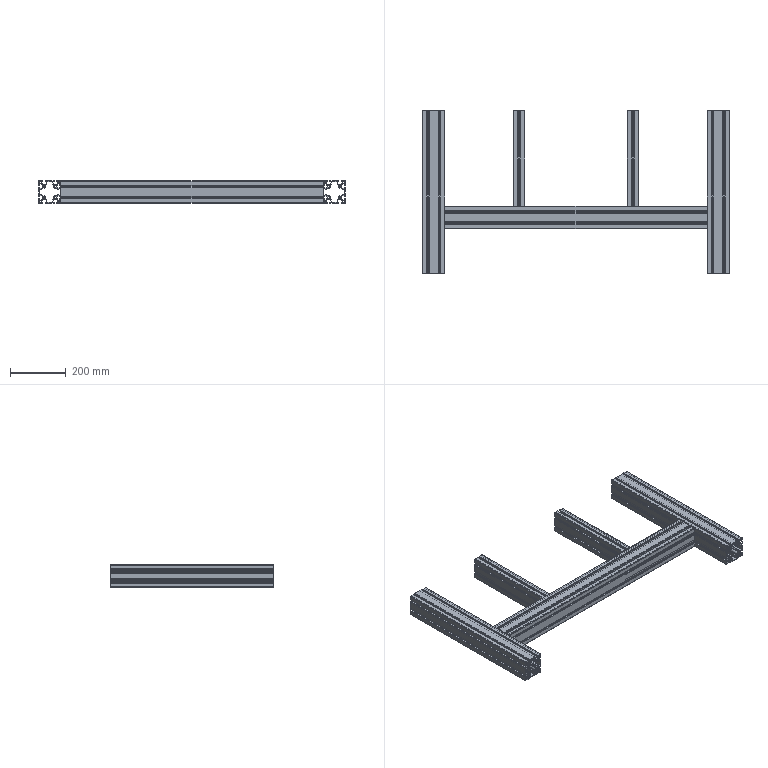Part | SolidWorks | features BaseBody 5 | 5 solids | 638 faces | box 1100 x 583 x 80 mm | volume 4144887 mm3 | plane 462 | cylinder 176 | commonest cylinder face diameters 20.04 x72 8 x40 6.8 x32 3 x20 12 x12